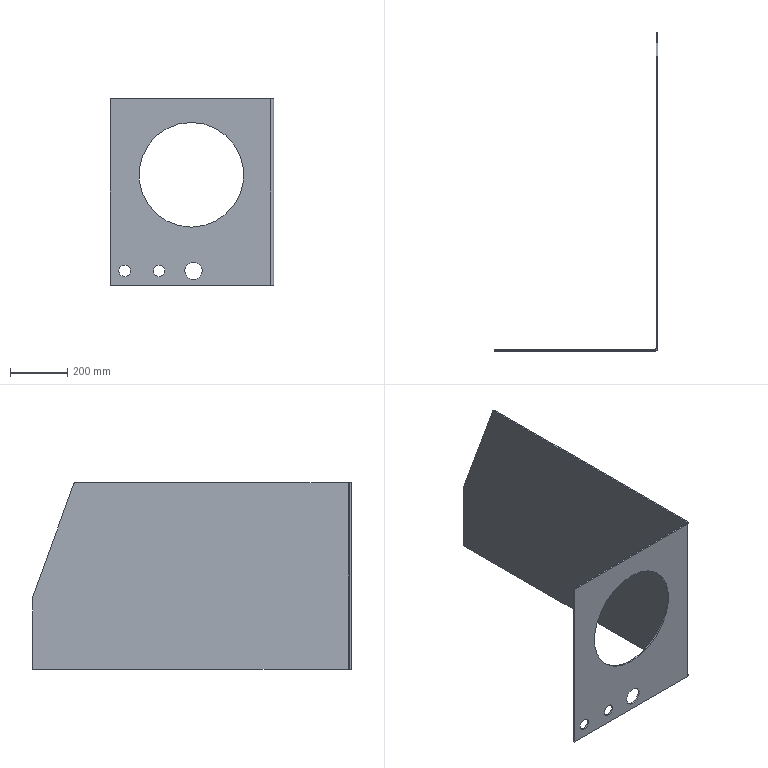Part | SolidWorks | features ICE 2, Fillet 1, FlatPattern 1, SMBaseFlange 1, SheetMetal 1, UnFold 1 | 1 solid | 25 faces | box 570.5 x 1110 x 651 mm | volume 4749925 mm3 | plane 13 | cylinder 12 | commonest cylinder face diameters 40 x4 12 x3 60 x2 365 x2 22 x1
STEP:
#1=CARTESIAN_POINT('',(50.5,5.,-295.));
#2=VERTEX_POINT('',#1);
#3=CARTESIAN_POINT('',(50.5,5.,-255.));
#4=VERTEX_POINT('',#3);
#5=CARTESIAN_POINT('',(50.5,5.,-275.));
#6=DIRECTION('',(0.,1.,0.));
#7=DIRECTION('',(0.,0.,1.));
#8=AXIS2_PLACEMENT_3D('',#5,#6,#7);
#9=CIRCLE('',#8,20.);
#10=EDGE_CURVE('',#2,#4,#9,.T.);
#11=ORIENTED_EDGE('',*,*,#10,.T.);
#12=CARTESIAN_POINT('',(50.5,0.,-255.));
#13=VERTEX_POINT('',#12);
#14=CARTESIAN_POINT('',(50.5,1110.5,-255.));
#15=DIRECTION('',(0.,-1.,0.));
#16=VECTOR('',#15,1000.);
#17=LINE('',#14,#16);
#18=EDGE_CURVE('',#4,#13,#17,.T.);
#19=ORIENTED_EDGE('',*,*,#18,.T.);
#20=CARTESIAN_POINT('',(50.5,0.,-295.));
#21=VERTEX_POINT('',#20);
#22=CARTESIAN_POINT('',(50.5,0.,-275.));
#23=DIRECTION('',(0.,-1.,0.));
#24=DIRECTION('',(0.,0.,-1.));
#25=AXIS2_PLACEMENT_3D('',#22,#23,#24);
#26=CIRCLE('',#25,20.);
#27=EDGE_CURVE('',#13,#21,#26,.T.);
#28=ORIENTED_EDGE('',*,*,#27,.T.);
#29=CARTESIAN_POINT('',(50.5,1110.5,-295.));
#30=DIRECTION('',(0.,-1.,0.));
#31=VECTOR('',#30,1000.);
#32=LINE('',#29,#31);
#33=EDGE_CURVE('',#2,#21,#32,.T.);
#34=ORIENTED_EDGE('',*,*,#33,.F.);
#35=EDGE_LOOP('',(#11,#19,#28,#34));
#36=FACE_OUTER_BOUND('',#35,.T.);
#37=CARTESIAN_POINT('',(50.5,1110.5,-275.));
#38=DIRECTION('',(0.,-1.,0.));
#39=DIRECTION('',(0.,0.,-1.));
#40=AXIS2_PLACEMENT_3D('',#37,#38,#39);
#41=CYLINDRICAL_SURFACE('',#40,20.);
#42=ADVANCED_FACE('',(#36),#41,.F.);
#43=CARTESIAN_POINT('',(170.5,5.,-295.));
#44=VERTEX_POINT('',#43);
#45=CARTESIAN_POINT('',(170.5,5.,-255.));
#46=VERTEX_POINT('',#45);
#47=CARTESIAN_POINT('',(170.5,5.,-275.));
#48=DIRECTION('',(0.,1.,0.));
#49=DIRECTION('',(0.,0.,1.));
#50=AXIS2_PLACEMENT_3D('',#47,#48,#49);
#51=CIRCLE('',#50,20.);
#52=EDGE_CURVE('',#44,#46,#51,.T.);
#53=ORIENTED_EDGE('',*,*,#52,.T.);
#54=CARTESIAN_POINT('',(170.5,0.,-255.));
#55=VERTEX_POINT('',#54);
#56=CARTESIAN_POINT('',(170.5,1110.5,-255.));
#57=DIRECTION('',(0.,-1.,0.));
#58=VECTOR('',#57,1000.);
#59=LINE('',#56,#58);
#60=EDGE_CURVE('',#46,#55,#59,.T.);
#61=ORIENTED_EDGE('',*,*,#60,.T.);
#62=CARTESIAN_POINT('',(170.5,0.,-295.));
#63=VERTEX_POINT('',#62);
#64=CARTESIAN_POINT('',(170.5,0.,-275.));
#65=DIRECTION('',(0.,-1.,0.));
#66=DIRECTION('',(0.,0.,-1.));
#67=AXIS2_PLACEMENT_3D('',#64,#65,#66);
#68=CIRCLE('',#67,20.);
#69=EDGE_CURVE('',#55,#63,#68,.T.);
#70=ORIENTED_EDGE('',*,*,#69,.T.);
#71=CARTESIAN_POINT('',(170.5,1110.5,-295.));
#72=DIRECTION('',(0.,-1.,0.));
#73=VECTOR('',#72,1000.);
#74=LINE('',#71,#73);
#75=EDGE_CURVE('',#44,#63,#74,.T.);
#76=ORIENTED_EDGE('',*,*,#75,.F.);
#77=EDGE_LOOP('',(#53,#61,#70,#76));
#78=FACE_OUTER_BOUND('',#77,.T.);
#79=CARTESIAN_POINT('',(170.5,1110.5,-275.));
#80=DIRECTION('',(0.,-1.,0.));
#81=DIRECTION('',(0.,0.,-1.));
#82=AXIS2_PLACEMENT_3D('',#79,#80,#81);
#83=CYLINDRICAL_SURFACE('',#82,20.);
#84=ADVANCED_FACE('',(#78),#83,.F.);
#85=CARTESIAN_POINT('',(290.5,5.,-305.));
#86=VERTEX_POINT('',#85);
#87=CARTESIAN_POINT('',(290.5,5.,-245.));
#88=VERTEX_POINT('',#87);
#89=CARTESIAN_POINT('',(290.5,5.,-275.));
#90=DIRECTION('',(0.,1.,0.));
#91=DIRECTION('',(0.,0.,1.));
#92=AXIS2_PLACEMENT_3D('',#89,#90,#91);
#93=CIRCLE('',#92,30.);
#94=EDGE_CURVE('',#86,#88,#93,.T.);
#95=ORIENTED_EDGE('',*,*,#94,.T.);
#96=CARTESIAN_POINT('',(290.5,0.,-245.));
#97=VERTEX_POINT('',#96);
#98=CARTESIAN_POINT('',(290.5,1110.5,-245.));
#99=DIRECTION('',(0.,-1.,0.));
#100=VECTOR('',#99,1000.);
#101=LINE('',#98,#100);
#102=EDGE_CURVE('',#88,#97,#101,.T.);
#103=ORIENTED_EDGE('',*,*,#102,.T.);
#104=CARTESIAN_POINT('',(290.5,0.,-305.));
#105=VERTEX_POINT('',#104);
#106=CARTESIAN_POINT('',(290.5,0.,-275.));
#107=DIRECTION('',(0.,-1.,0.));
#108=DIRECTION('',(0.,0.,-1.));
#109=AXIS2_PLACEMENT_3D('',#106,#107,#108);
#110=CIRCLE('',#109,30.);
#111=EDGE_CURVE('',#97,#105,#110,.T.);
#112=ORIENTED_EDGE('',*,*,#111,.T.);
#113=CARTESIAN_POINT('',(290.5,1110.5,-305.));
#114=DIRECTION('',(0.,-1.,0.));
#115=VECTOR('',#114,1000.);
#116=LINE('',#113,#115);
#117=EDGE_CURVE('',#86,#105,#116,.T.);
#118=ORIENTED_EDGE('',*,*,#117,.F.);
#119=EDGE_LOOP('',(#95,#103,#112,#118));
#120=FACE_OUTER_BOUND('',#119,.T.);
#121=CARTESIAN_POINT('',(290.5,1110.5,-275.));
#122=DIRECTION('',(0.,-1.,0.));
#123=DIRECTION('',(0.,0.,-1.));
#124=AXIS2_PLACEMENT_3D('',#121,#122,#123);
#125=CYLINDRICAL_SURFACE('',#124,30.);
#126=ADVANCED_FACE('',(#120),#125,.F.);
#127=CARTESIAN_POINT('',(283.,5.,-122.5));
#128=VERTEX_POINT('',#127);
#129=CARTESIAN_POINT('',(283.,5.,242.5));
#130=VERTEX_POINT('',#129);
#131=CARTESIAN_POINT('',(283.,5.,60.));
#132=DIRECTION('',(0.,1.,0.));
#133=DIRECTION('',(0.,0.,1.));
#134=AXIS2_PLACEMENT_3D('',#131,#132,#133);
#135=CIRCLE('',#134,182.5);
#136=EDGE_CURVE('',#128,#130,#135,.T.);
#137=ORIENTED_EDGE('',*,*,#136,.T.);
#138=CARTESIAN_POINT('',(283.,0.,242.5));
#139=VERTEX_POINT('',#138);
#140=CARTESIAN_POINT('',(283.,1110.5,242.5));
#141=DIRECTION('',(0.,-1.,0.));
#142=VECTOR('',#141,1000.);
#143=LINE('',#140,#142);
#144=EDGE_CURVE('',#130,#139,#143,.T.);
#145=ORIENTED_EDGE('',*,*,#144,.T.);
#146=CARTESIAN_POINT('',(283.,0.,-122.5));
#147=VERTEX_POINT('',#146);
#148=CARTESIAN_POINT('',(283.,0.,60.));
#149=DIRECTION('',(0.,-1.,0.));
#150=DIRECTION('',(0.,0.,-1.));
#151=AXIS2_PLACEMENT_3D('',#148,#149,#150);
#152=CIRCLE('',#151,182.5);
#153=EDGE_CURVE('',#139,#147,#152,.T.);
#154=ORIENTED_EDGE('',*,*,#153,.T.);
#155=CARTESIAN_POINT('',(283.,1110.5,-122.5));
#156=DIRECTION('',(0.,-1.,0.));
#157=VECTOR('',#156,1000.);
#158=LINE('',#155,#157);
#159=EDGE_CURVE('',#128,#147,#158,.T.);
#160=ORIENTED_EDGE('',*,*,#159,.F.);
#161=EDGE_LOOP('',(#137,#145,#154,#160));
#162=FACE_OUTER_BOUND('',#161,.T.);
#163=CARTESIAN_POINT('',(283.,1110.5,60.));
#164=DIRECTION('',(0.,-1.,0.));
#165=DIRECTION('',(0.,0.,-1.));
#166=AXIS2_PLACEMENT_3D('',#163,#164,#165);
#167=CYLINDRICAL_SURFACE('',#166,182.5);
#168=ADVANCED_FACE('',(#162),#167,.F.);
#169=CARTESIAN_POINT('',(559.5,0.,325.5));
#170=VERTEX_POINT('',#169);
#171=CARTESIAN_POINT('',(559.5,5.,325.5));
#172=VERTEX_POINT('',#171);
#173=CARTESIAN_POINT('',(559.5,0.,325.5));
#174=DIRECTION('',(0.,1.,0.));
#175=VECTOR('',#174,1000.);
#176=LINE('',#173,#175);
#177=EDGE_CURVE('',#170,#172,#176,.T.);
#178=ORIENTED_EDGE('',*,*,#177,.F.);
#179=CARTESIAN_POINT('',(570.5,11.,325.5));
#180=VERTEX_POINT('',#179);
#181=CARTESIAN_POINT('',(559.5,11.,325.5));
#182=DIRECTION('',(0.,0.,1.));
#183=DIRECTION('',(-1.,0.,0.));
#184=AXIS2_PLACEMENT_3D('',#181,#182,#183);
#185=CIRCLE('',#184,11.);
#186=EDGE_CURVE('',#170,#180,#185,.T.);
#187=ORIENTED_EDGE('',*,*,#186,.T.);
#188=CARTESIAN_POINT('',(565.5,11.,325.5));
#189=VERTEX_POINT('',#188);
#190=CARTESIAN_POINT('',(565.5,11.,325.5));
#191=DIRECTION('',(1.,0.,0.));
#192=VECTOR('',#191,1000.);
#193=LINE('',#190,#192);
#194=EDGE_CURVE('',#189,#180,#193,.T.);
#195=ORIENTED_EDGE('',*,*,#194,.F.);
#196=CARTESIAN_POINT('',(559.5,11.,325.5));
#197=DIRECTION('',(0.,0.,1.));
#198=DIRECTION('',(1.,0.,0.));
#199=AXIS2_PLACEMENT_3D('',#196,#197,#198);
#200=CIRCLE('',#199,6.);
#201=EDGE_CURVE('',#172,#189,#200,.T.);
#202=ORIENTED_EDGE('',*,*,#201,.F.);
#203=EDGE_LOOP('',(#178,#187,#195,#202));
#204=FACE_OUTER_BOUND('',#203,.T.);
#205=CARTESIAN_POINT('',(559.5,0.,325.5));
#206=DIRECTION('',(0.,0.,1.));
#207=DIRECTION('',(1.,0.,0.));
#208=AXIS2_PLACEMENT_3D('',#205,#206,#207);
#209=PLANE('',#208);
#210=ADVANCED_FACE('',(#204),#209,.T.);
#211=CARTESIAN_POINT('',(0.,0.,325.5));
#212=VERTEX_POINT('',#211);
#213=CARTESIAN_POINT('',(0.,0.,325.5));
#214=DIRECTION('',(1.,0.,0.));
#215=VECTOR('',#214,1000.);
#216=LINE('',#213,#215);
#217=EDGE_CURVE('',#212,#170,#216,.T.);
#218=ORIENTED_EDGE('',*,*,#217,.T.);
#219=ORIENTED_EDGE('',*,*,#177,.T.);
#220=CARTESIAN_POINT('',(0.,5.,325.5));
#221=VERTEX_POINT('',#220);
#222=CARTESIAN_POINT('',(0.,5.,325.5));
#223=DIRECTION('',(1.,0.,0.));
#224=VECTOR('',#223,1000.);
#225=LINE('',#222,#224);
#226=EDGE_CURVE('',#221,#172,#225,.T.);
#227=ORIENTED_EDGE('',*,*,#226,.F.);
#228=CARTESIAN_POINT('',(0.,0.,325.5));
#229=DIRECTION('',(0.,1.,0.));
#230=VECTOR('',#229,1000.);
#231=LINE('',#228,#230);
#232=EDGE_CURVE('',#212,#221,#231,.T.);
#233=ORIENTED_EDGE('',*,*,#232,.F.);
#234=EDGE_LOOP('',(#218,#219,#227,#233));
#235=FACE_OUTER_BOUND('',#234,.T.);
#236=CARTESIAN_POINT('',(565.5,11.,325.5));
#237=DIRECTION('',(0.,0.,1.));
#238=DIRECTION('',(1.,0.,0.));
#239=AXIS2_PLACEMENT_3D('',#236,#237,#238);
#240=PLANE('',#239);
#241=ADVANCED_FACE('',(#235),#240,.T.);
#242=CARTESIAN_POINT('',(570.5,11.,-325.5));
#243=VERTEX_POINT('',#242);
#244=CARTESIAN_POINT('',(565.5,11.,-325.5));
#245=VERTEX_POINT('',#244);
#246=CARTESIAN_POINT('',(570.5,11.,-325.5));
#247=DIRECTION('',(-1.,0.,0.));
#248=VECTOR('',#247,1000.);
#249=LINE('',#246,#248);
#250=EDGE_CURVE('',#243,#245,#249,.T.);
#251=ORIENTED_EDGE('',*,*,#250,.F.);
#252=CARTESIAN_POINT('',(559.5,0.,-325.5));
#253=VERTEX_POINT('',#252);
#254=CARTESIAN_POINT('',(559.5,11.,-325.5));
#255=DIRECTION('',(0.,0.,1.));
#256=DIRECTION('',(-1.,0.,0.));
#257=AXIS2_PLACEMENT_3D('',#254,#255,#256);
#258=CIRCLE('',#257,11.);
#259=EDGE_CURVE('',#253,#243,#258,.T.);
#260=ORIENTED_EDGE('',*,*,#259,.F.);
#261=CARTESIAN_POINT('',(559.5,5.,-325.5));
#262=VERTEX_POINT('',#261);
#263=CARTESIAN_POINT('',(559.5,5.,-325.5));
#264=DIRECTION('',(0.,-1.,0.));
#265=VECTOR('',#264,1000.);
#266=LINE('',#263,#265);
#267=EDGE_CURVE('',#262,#253,#266,.T.);
#268=ORIENTED_EDGE('',*,*,#267,.F.);
#269=CARTESIAN_POINT('',(559.5,11.,-325.5));
#270=DIRECTION('',(0.,0.,1.));
#271=DIRECTION('',(1.,0.,0.));
#272=AXIS2_PLACEMENT_3D('',#269,#270,#271);
#273=CIRCLE('',#272,6.);
#274=EDGE_CURVE('',#262,#245,#273,.T.);
#275=ORIENTED_EDGE('',*,*,#274,.T.);
#276=EDGE_LOOP('',(#251,#260,#268,#275));
#277=FACE_OUTER_BOUND('',#276,.T.);
#278=CARTESIAN_POINT('',(570.5,11.,-325.5));
#279=DIRECTION('',(0.,0.,-1.));
#280=DIRECTION('',(-1.,0.,0.));
#281=AXIS2_PLACEMENT_3D('',#278,#279,#280);
#282=PLANE('',#281);
#283=ADVANCED_FACE('',(#277),#282,.T.);
#284=CARTESIAN_POINT('',(570.5,1110.5,-325.5));
#285=VERTEX_POINT('',#284);
#286=CARTESIAN_POINT('',(570.5,0.,-325.5));
#287=DIRECTION('',(0.,1.,0.));
#288=VECTOR('',#287,1000.);
#289=LINE('',#286,#288);
#290=EDGE_CURVE('',#243,#285,#289,.T.);
#291=ORIENTED_EDGE('',*,*,#290,.F.);
#292=ORIENTED_EDGE('',*,*,#250,.T.);
#293=CARTESIAN_POINT('',(565.5,1110.5,-325.5));
#294=VERTEX_POINT('',#293);
#295=CARTESIAN_POINT('',(565.5,0.,-325.5));
#296=DIRECTION('',(0.,1.,0.));
#297=VECTOR('',#296,1000.);
#298=LINE('',#295,#297);
#299=EDGE_CURVE('',#245,#294,#298,.T.);
#300=ORIENTED_EDGE('',*,*,#299,.T.);
#301=CARTESIAN_POINT('',(565.5,1110.5,-325.5));
#302=DIRECTION('',(1.,0.,0.));
#303=VECTOR('',#302,1000.);
#304=LINE('',#301,#303);
#305=EDGE_CURVE('',#294,#285,#304,.T.);
#306=ORIENTED_EDGE('',*,*,#305,.T.);
#307=EDGE_LOOP('',(#291,#292,#300,#306));
#308=FACE_OUTER_BOUND('',#307,.T.);
#309=CARTESIAN_POINT('',(559.5,5.,-325.5));
#310=DIRECTION('',(0.,0.,-1.));
#311=DIRECTION('',(-1.,0.,0.));
#312=AXIS2_PLACEMENT_3D('',#309,#310,#311);
#313=PLANE('',#312);
#314=ADVANCED_FACE('',(#308),#313,.T.);
#315=CARTESIAN_POINT('',(570.5,1110.5,-72.938));
#316=VERTEX_POINT('',#315);
#317=CARTESIAN_POINT('',(570.5,1110.5,325.5));
#318=DIRECTION('',(0.,0.,-1.));
#319=VECTOR('',#318,1000.);
#320=LINE('',#317,#319);
#321=EDGE_CURVE('',#316,#285,#320,.T.);
#322=ORIENTED_EDGE('',*,*,#321,.F.);
#323=CARTESIAN_POINT('',(570.5,1110.138,-70.886));
#324=VERTEX_POINT('',#323);
#325=CARTESIAN_POINT('',(570.5,1104.5,-72.938));
#326=DIRECTION('',(1.,0.,0.));
#327=DIRECTION('',(0.,0.,1.));
#328=AXIS2_PLACEMENT_3D('',#325,#326,#327);
#329=CIRCLE('',#328,6.);
#330=EDGE_CURVE('',#316,#324,#329,.T.);
#331=ORIENTED_EDGE('',*,*,#330,.T.);
#332=CARTESIAN_POINT('',(570.5,967.302,321.552));
#333=VERTEX_POINT('',#332);
#334=CARTESIAN_POINT('',(570.5,1110.5,-71.88));
#335=DIRECTION('',(0.,0.342,-0.9397));
#336=VECTOR('',#335,1000.);
#337=LINE('',#334,#336);
#338=EDGE_CURVE('',#333,#324,#337,.T.);
#339=ORIENTED_EDGE('',*,*,#338,.F.);
#340=CARTESIAN_POINT('',(570.5,961.664,325.5));
#341=VERTEX_POINT('',#340);
#342=CARTESIAN_POINT('',(570.5,961.664,319.5));
#343=DIRECTION('',(1.,0.,0.));
#344=DIRECTION('',(0.,0.,1.));
#345=AXIS2_PLACEMENT_3D('',#342,#343,#344);
#346=CIRCLE('',#345,6.);
#347=EDGE_CURVE('',#333,#341,#346,.T.);
#348=ORIENTED_EDGE('',*,*,#347,.T.);
#349=CARTESIAN_POINT('',(570.5,0.,325.5));
#350=DIRECTION('',(0.,1.,0.));
#351=VECTOR('',#350,1000.);
#352=LINE('',#349,#351);
#353=EDGE_CURVE('',#180,#341,#352,.T.);
#354=ORIENTED_EDGE('',*,*,#353,.F.);
#355=CARTESIAN_POINT('',(570.5,11.,325.5));
#356=DIRECTION('',(0.,0.,-1.));
#357=VECTOR('',#356,1000.);
#358=LINE('',#355,#357);
#359=EDGE_CURVE('',#180,#243,#358,.T.);
#360=ORIENTED_EDGE('',*,*,#359,.T.);
#361=ORIENTED_EDGE('',*,*,#290,.T.);
#362=EDGE_LOOP('',(#322,#331,#339,#348,#354,#360,#361));
#363=FACE_OUTER_BOUND('',#362,.T.);
#364=CARTESIAN_POINT('',(570.5,0.,325.5));
#365=DIRECTION('',(-1.,0.,0.));
#366=DIRECTION('',(0.,0.,1.));
#367=AXIS2_PLACEMENT_3D('',#364,#365,#366);
#368=PLANE('',#367);
#369=ADVANCED_FACE('',(#363),#368,.F.);
#370=CARTESIAN_POINT('',(565.5,1110.5,-72.938));
#371=VERTEX_POINT('',#370);
#372=CARTESIAN_POINT('',(565.5,1110.5,325.5));
#373=DIRECTION('',(0.,0.,-1.));
#374=VECTOR('',#373,1000.);
#375=LINE('',#372,#374);
#376=EDGE_CURVE('',#371,#294,#375,.T.);
#377=ORIENTED_EDGE('',*,*,#376,.F.);
#378=CARTESIAN_POINT('',(570.5,1110.5,-72.938));
#379=DIRECTION('',(1.,0.,0.));
#380=VECTOR('',#379,1000.);
#381=LINE('',#378,#380);
#382=EDGE_CURVE('',#371,#316,#381,.T.);
#383=ORIENTED_EDGE('',*,*,#382,.T.);
#384=ORIENTED_EDGE('',*,*,#321,.T.);
#385=ORIENTED_EDGE('',*,*,#305,.F.);
#386=EDGE_LOOP('',(#377,#383,#384,#385));
#387=FACE_OUTER_BOUND('',#386,.T.);
#388=CARTESIAN_POINT('',(565.5,1110.5,325.5));
#389=DIRECTION('',(0.,1.,0.));
#390=DIRECTION('',(0.,0.,1.));
#391=AXIS2_PLACEMENT_3D('',#388,#389,#390);
#392=PLANE('',#391);
#393=ADVANCED_FACE('',(#387),#392,.T.);
#394=CARTESIAN_POINT('',(565.5,1110.138,-70.886));
#395=VERTEX_POINT('',#394);
#396=CARTESIAN_POINT('',(565.5,967.302,321.552));
#397=VERTEX_POINT('',#396);
#398=CARTESIAN_POINT('',(565.5,852.881,635.923));
#399=DIRECTION('',(0.,-0.342,0.9397));
#400=VECTOR('',#399,1000.);
#401=LINE('',#398,#400);
#402=EDGE_CURVE('',#395,#397,#401,.T.);
#403=ORIENTED_EDGE('',*,*,#402,.F.);
#404=CARTESIAN_POINT('',(565.5,1104.5,-72.938));
#405=DIRECTION('',(-1.,0.,0.));
#406=DIRECTION('',(0.,0.,1.));
#407=AXIS2_PLACEMENT_3D('',#404,#405,#406);
#408=CIRCLE('',#407,6.);
#409=EDGE_CURVE('',#395,#371,#408,.T.);
#410=ORIENTED_EDGE('',*,*,#409,.T.);
#411=ORIENTED_EDGE('',*,*,#376,.T.);
#412=ORIENTED_EDGE('',*,*,#299,.F.);
#413=CARTESIAN_POINT('',(565.5,11.,325.5));
#414=DIRECTION('',(0.,0.,-1.));
#415=VECTOR('',#414,1000.);
#416=LINE('',#413,#415);
#417=EDGE_CURVE('',#189,#245,#416,.T.);
#418=ORIENTED_EDGE('',*,*,#417,.F.);
#419=CARTESIAN_POINT('',(565.5,961.664,325.5));
#420=VERTEX_POINT('',#419);
#421=CARTESIAN_POINT('',(565.5,0.,325.5));
#422=DIRECTION('',(0.,1.,0.));
#423=VECTOR('',#422,1000.);
#424=LINE('',#421,#423);
#425=EDGE_CURVE('',#189,#420,#424,.T.);
#426=ORIENTED_EDGE('',*,*,#425,.T.);
#427=CARTESIAN_POINT('',(565.5,961.664,319.5));
#428=DIRECTION('',(-1.,0.,0.));
#429=DIRECTION('',(0.,0.,1.));
#430=AXIS2_PLACEMENT_3D('',#427,#428,#429);
#431=CIRCLE('',#430,6.);
#432=EDGE_CURVE('',#420,#397,#431,.T.);
#433=ORIENTED_EDGE('',*,*,#432,.T.);
#434=EDGE_LOOP('',(#403,#410,#411,#412,#418,#426,#433));
#435=FACE_OUTER_BOUND('',#434,.T.);
#436=CARTESIAN_POINT('',(565.5,0.,325.5));
#437=DIRECTION('',(-1.,0.,0.));
#438=DIRECTION('',(0.,0.,1.));
#439=AXIS2_PLACEMENT_3D('',#436,#437,#438);
#440=PLANE('',#439);
#441=ADVANCED_FACE('',(#435),#440,.T.);
#442=ORIENTED_EDGE('',*,*,#274,.F.);
#443=CARTESIAN_POINT('',(559.5,5.,325.5));
#444=DIRECTION('',(0.,0.,-1.));
#445=VECTOR('',#444,1000.);
#446=LINE('',#443,#445);
#447=EDGE_CURVE('',#172,#262,#446,.T.);
#448=ORIENTED_EDGE('',*,*,#447,.F.);
#449=ORIENTED_EDGE('',*,*,#201,.T.);
#450=ORIENTED_EDGE('',*,*,#417,.T.);
#451=EDGE_LOOP('',(#442,#448,#449,#450));
#452=FACE_OUTER_BOUND('',#451,.T.);
#453=CARTESIAN_POINT('',(559.5,11.,325.5));
#454=DIRECTION('',(0.,0.,-1.));
#455=DIRECTION('',(-1.,0.,0.));
#456=AXIS2_PLACEMENT_3D('',#453,#454,#455);
#457=CYLINDRICAL_SURFACE('',#456,6.);
#458=ADVANCED_FACE('',(#452),#457,.F.);
#459=ORIENTED_EDGE('',*,*,#10,.F.);
#460=CARTESIAN_POINT('',(50.5,5.,-275.));
#461=DIRECTION('',(0.,1.,0.));
#462=DIRECTION('',(0.,0.,1.));
#463=AXIS2_PLACEMENT_3D('',#460,#461,#462);
#464=CIRCLE('',#463,20.);
#465=EDGE_CURVE('',#4,#2,#464,.T.);
#466=ORIENTED_EDGE('',*,*,#465,.F.);
#467=EDGE_LOOP('',(#459,#466));
#468=FACE_BOUND('',#467,.T.);
#469=ORIENTED_EDGE('',*,*,#52,.F.);
#470=CARTESIAN_POINT('',(170.5,5.,-275.));
#471=DIRECTION('',(0.,1.,0.));
#472=DIRECTION('',(0.,0.,1.));
#473=AXIS2_PLACEMENT_3D('',#470,#471,#472);
#474=CIRCLE('',#473,20.);
#475=EDGE_CURVE('',#46,#44,#474,.T.);
#476=ORIENTED_EDGE('',*,*,#475,.F.);
#477=EDGE_LOOP('',(#469,#476));
#478=FACE_BOUND('',#477,.T.);
#479=ORIENTED_EDGE('',*,*,#94,.F.);
#480=CARTESIAN_POINT('',(290.5,5.,-275.));
#481=DIRECTION('',(0.,1.,0.));
#482=DIRECTION('',(0.,0.,1.));
#483=AXIS2_PLACEMENT_3D('',#480,#481,#482);
#484=CIRCLE('',#483,30.);
#485=EDGE_CURVE('',#88,#86,#484,.T.);
#486=ORIENTED_EDGE('',*,*,#485,.F.);
#487=EDGE_LOOP('',(#479,#486));
#488=FACE_BOUND('',#487,.T.);
#489=ORIENTED_EDGE('',*,*,#136,.F.);
#490=CARTESIAN_POINT('',(283.,5.,60.));
#491=DIRECTION('',(0.,1.,0.));
#492=DIRECTION('',(0.,0.,1.));
#493=AXIS2_PLACEMENT_3D('',#490,#491,#492);
#494=CIRCLE('',#493,182.5);
#495=EDGE_CURVE('',#130,#128,#494,.T.);
#496=ORIENTED_EDGE('',*,*,#495,.F.);
#497=EDGE_LOOP('',(#489,#496));
#498=FACE_BOUND('',#497,.T.);
#499=CARTESIAN_POINT('',(0.,5.,-325.5));
#500=VERTEX_POINT('',#499);
#501=CARTESIAN_POINT('',(0.,5.,-325.5));
#502=DIRECTION('',(1.,0.,0.));
#503=VECTOR('',#502,1000.);
#504=LINE('',#501,#503);
#505=EDGE_CURVE('',#500,#262,#504,.T.);
#506=ORIENTED_EDGE('',*,*,#505,.F.);
#507=CARTESIAN_POINT('',(0.,5.,325.5));
#508=DIRECTION('',(0.,0.,-1.));
#509=VECTOR('',#508,1000.);
#510=LINE('',#507,#509);
#511=EDGE_CURVE('',#221,#500,#510,.T.);
#512=ORIENTED_EDGE('',*,*,#511,.F.);
#513=ORIENTED_EDGE('',*,*,#226,.T.);
#514=ORIENTED_EDGE('',*,*,#447,.T.);
#515=EDGE_LOOP('',(#506,#512,#513,#514));
#516=FACE_OUTER_BOUND('',#515,.T.);
#517=CARTESIAN_POINT('',(0.,5.,325.5));
#518=DIRECTION('',(0.,1.,0.));
#519=DIRECTION('',(0.,0.,1.));
#520=AXIS2_PLACEMENT_3D('',#517,#518,#519);
#521=PLANE('',#520);
#522=ADVANCED_FACE('',(#468,#478,#488,#498,#516),#521,.T.);
#523=CARTESIAN_POINT('',(0.,0.,-325.5));
#524=VERTEX_POINT('',#523);
#525=CARTESIAN_POINT('',(0.,0.,-325.5));
#526=DIRECTION('',(0.,1.,0.));
#527=VECTOR('',#526,1000.);
#528=LINE('',#525,#527);
#529=EDGE_CURVE('',#524,#500,#528,.T.);
#530=ORIENTED_EDGE('',*,*,#529,.F.);
#531=CARTESIAN_POINT('',(0.,0.,325.5));
#532=DIRECTION('',(0.,0.,-1.));
#533=VECTOR('',#532,1000.);
#534=LINE('',#531,#533);
#535=EDGE_CURVE('',#212,#524,#534,.T.);
#536=ORIENTED_EDGE('',*,*,#535,.F.);
#537=ORIENTED_EDGE('',*,*,#232,.T.);
#538=ORIENTED_EDGE('',*,*,#511,.T.);
#539=EDGE_LOOP('',(#530,#536,#537,#538));
#540=FACE_OUTER_BOUND('',#539,.T.);
#541=CARTESIAN_POINT('',(0.,0.,325.5));
#542=DIRECTION('',(-1.,0.,0.));
#543=DIRECTION('',(0.,0.,1.));
#544=AXIS2_PLACEMENT_3D('',#541,#542,#543);
#545=PLANE('',#544);
#546=ADVANCED_FACE('',(#540),#545,.T.);
#547=CARTESIAN_POINT('',(50.5,0.,-275.));
#548=DIRECTION('',(0.,-1.,0.));
#549=DIRECTION('',(0.,0.,-1.));
#550=AXIS2_PLACEMENT_3D('',#547,#548,#549);
#551=CIRCLE('',#550,20.);
#552=EDGE_CURVE('',#21,#13,#551,.T.);
#553=ORIENTED_EDGE('',*,*,#552,.F.);
#554=ORIENTED_EDGE('',*,*,#27,.F.);
#555=EDGE_LOOP('',(#553,#554));
#556=FACE_BOUND('',#555,.T.);
#557=CARTESIAN_POINT('',(170.5,0.,-275.));
#558=DIRECTION('',(0.,-1.,0.));
#559=DIRECTION('',(0.,0.,-1.));
#560=AXIS2_PLACEMENT_3D('',#557,#558,#559);
#561=CIRCLE('',#560,20.);
#562=EDGE_CURVE('',#63,#55,#561,.T.);
#563=ORIENTED_EDGE('',*,*,#562,.F.);
#564=ORIENTED_EDGE('',*,*,#69,.F.);
#565=EDGE_LOOP('',(#563,#564));
#566=FACE_BOUND('',#565,.T.);
#567=CARTESIAN_POINT('',(290.5,0.,-275.));
#568=DIRECTION('',(0.,-1.,0.));
#569=DIRECTION('',(0.,0.,-1.));
#570=AXIS2_PLACEMENT_3D('',#567,#568,#569);
#571=CIRCLE('',#570,30.);
#572=EDGE_CURVE('',#105,#97,#571,.T.);
#573=ORIENTED_EDGE('',*,*,#572,.F.);
#574=ORIENTED_EDGE('',*,*,#111,.F.);
#575=EDGE_LOOP('',(#573,#574));
#576=FACE_BOUND('',#575,.T.);
#577=CARTESIAN_POINT('',(283.,0.,60.));
#578=DIRECTION('',(0.,-1.,0.));
#579=DIRECTION('',(0.,0.,-1.));
#580=AXIS2_PLACEMENT_3D('',#577,#578,#579);
#581=CIRCLE('',#580,182.5);
#582=EDGE_CURVE('',#147,#139,#581,.T.);
#583=ORIENTED_EDGE('',*,*,#582,.F.);
#584=ORIENTED_EDGE('',*,*,#153,.F.);
#585=EDGE_LOOP('',(#583,#584));
#586=FACE_BOUND('',#585,.T.);
#587=CARTESIAN_POINT('',(0.,0.,-325.5));
#588=DIRECTION('',(1.,0.,0.));
#589=VECTOR('',#588,1000.);
#590=LINE('',#587,#589);
#591=EDGE_CURVE('',#524,#253,#590,.T.);
#592=ORIENTED_EDGE('',*,*,#591,.T.);
#593=CARTESIAN_POINT('',(559.5,0.,325.5));
#594=DIRECTION('',(0.,0.,-1.));
#595=VECTOR('',#594,1000.);
#596=LINE('',#593,#595);
#597=EDGE_CURVE('',#170,#253,#596,.T.);
#598=ORIENTED_EDGE('',*,*,#597,.F.);
#599=ORIENTED_EDGE('',*,*,#217,.F.);
#600=ORIENTED_EDGE('',*,*,#535,.T.);
#601=EDGE_LOOP('',(#592,#598,#599,#600));
#602=FACE_OUTER_BOUND('',#601,.T.);
#603=CARTESIAN_POINT('',(0.,0.,325.5));
#604=DIRECTION('',(0.,1.,0.));
#605=DIRECTION('',(0.,0.,1.));
#606=AXIS2_PLACEMENT_3D('',#603,#604,#605);
#607=PLANE('',#606);
#608=ADVANCED_FACE('',(#556,#566,#576,#586,#602),#607,.F.);
#609=ORIENTED_EDGE('',*,*,#259,.T.);
#610=ORIENTED_EDGE('',*,*,#359,.F.);
#611=ORIENTED_EDGE('',*,*,#186,.F.);
#612=ORIENTED_EDGE('',*,*,#597,.T.);
#613=EDGE_LOOP('',(#609,#610,#611,#612));
#614=FACE_OUTER_BOUND('',#613,.T.);
#615=CARTESIAN_POINT('',(559.5,11.,325.5));
#616=DIRECTION('',(0.,0.,-1.));
#617=DIRECTION('',(-1.,0.,0.));
#618=AXIS2_PLACEMENT_3D('',#615,#616,#617);
#619=CYLINDRICAL_SURFACE('',#618,11.);
#620=ADVANCED_FACE('',(#614),#619,.T.);
#621=ORIENTED_EDGE('',*,*,#353,.T.);
#622=CARTESIAN_POINT('',(565.5,961.664,325.5));
#623=DIRECTION('',(-1.,0.,0.));
#624=VECTOR('',#623,1000.);
#625=LINE('',#622,#624);
#626=EDGE_CURVE('',#341,#420,#625,.T.);
#627=ORIENTED_EDGE('',*,*,#626,.T.);
#628=ORIENTED_EDGE('',*,*,#425,.F.);
#629=ORIENTED_EDGE('',*,*,#194,.T.);
#630=EDGE_LOOP('',(#621,#627,#628,#629));
#631=FACE_OUTER_BOUND('',#630,.T.);
#632=CARTESIAN_POINT('',(559.5,11.,325.5));
#633=DIRECTION('',(0.,0.,1.));
#634=DIRECTION('',(1.,0.,0.));
#635=AXIS2_PLACEMENT_3D('',#632,#633,#634);
#636=PLANE('',#635);
#637=ADVANCED_FACE('',(#631),#636,.T.);
#638=ORIENTED_EDGE('',*,*,#505,.T.);
#639=ORIENTED_EDGE('',*,*,#267,.T.);
#640=ORIENTED_EDGE('',*,*,#591,.F.);
#641=ORIENTED_EDGE('',*,*,#529,.T.);
#642=EDGE_LOOP('',(#638,#639,#640,#641));
#643=FACE_OUTER_BOUND('',#642,.T.);
#644=CARTESIAN_POINT('',(559.5,11.,-325.5));
#645=DIRECTION('',(0.,0.,1.));
#646=DIRECTION('',(1.,0.,0.));
#647=AXIS2_PLACEMENT_3D('',#644,#645,#646);
#648=PLANE('',#647);
#649=ADVANCED_FACE('',(#643),#648,.F.);
#650=ORIENTED_EDGE('',*,*,#338,.T.);
#651=CARTESIAN_POINT('',(565.5,1110.138,-70.886));
#652=DIRECTION('',(-1.,0.,0.));
#653=VECTOR('',#652,1000.);
#654=LINE('',#651,#653);
#655=EDGE_CURVE('',#324,#395,#654,.T.);
#656=ORIENTED_EDGE('',*,*,#655,.T.);
#657=ORIENTED_EDGE('',*,*,#402,.T.);
#658=CARTESIAN_POINT('',(570.5,967.302,321.552));
#659=DIRECTION('',(1.,0.,0.));
#660=VECTOR('',#659,1000.);
#661=LINE('',#658,#660);
#662=EDGE_CURVE('',#397,#333,#661,.T.);
#663=ORIENTED_EDGE('',*,*,#662,.T.);
#664=EDGE_LOOP('',(#650,#656,#657,#663));
#665=FACE_OUTER_BOUND('',#664,.T.);
#666=CARTESIAN_POINT('',(0.,1110.5,-71.88));
#667=DIRECTION('',(0.,-0.9397,-0.342));
#668=DIRECTION('',(0.,0.342,-0.9397));
#669=AXIS2_PLACEMENT_3D('',#666,#667,#668);
#670=PLANE('',#669);
#671=ADVANCED_FACE('',(#665),#670,.F.);
#672=ORIENTED_EDGE('',*,*,#409,.F.);
#673=ORIENTED_EDGE('',*,*,#655,.F.);
#674=ORIENTED_EDGE('',*,*,#330,.F.);
#675=ORIENTED_EDGE('',*,*,#382,.F.);
#676=EDGE_LOOP('',(#672,#673,#674,#675));
#677=FACE_OUTER_BOUND('',#676,.T.);
#678=CARTESIAN_POINT('',(565.5,1104.5,-72.938));
#679=DIRECTION('',(-1.,0.,0.));
#680=DIRECTION('',(0.,0.,1.));
#681=AXIS2_PLACEMENT_3D('',#678,#679,#680);
#682=CYLINDRICAL_SURFACE('',#681,6.);
#683=ADVANCED_FACE('',(#677),#682,.T.);
#684=ORIENTED_EDGE('',*,*,#432,.F.);
#685=ORIENTED_EDGE('',*,*,#626,.F.);
#686=ORIENTED_EDGE('',*,*,#347,.F.);
#687=ORIENTED_EDGE('',*,*,#662,.F.);
#688=EDGE_LOOP('',(#684,#685,#686,#687));
#689=FACE_OUTER_BOUND('',#688,.T.);
#690=CARTESIAN_POINT('',(0.,961.664,319.5));
#691=DIRECTION('',(-1.,0.,0.));
#692=DIRECTION('',(0.,0.,1.));
#693=AXIS2_PLACEMENT_3D('',#690,#691,#692);
#694=CYLINDRICAL_SURFACE('',#693,6.);
#695=ADVANCED_FACE('',(#689),#694,.T.);
#696=ORIENTED_EDGE('',*,*,#144,.F.);
#697=ORIENTED_EDGE('',*,*,#495,.T.);
#698=ORIENTED_EDGE('',*,*,#159,.T.);
#699=ORIENTED_EDGE('',*,*,#582,.T.);
#700=EDGE_LOOP('',(#696,#697,#698,#699));
#701=FACE_OUTER_BOUND('',#700,.T.);
#702=CARTESIAN_POINT('',(283.,1110.5,60.));
#703=DIRECTION('',(0.,-1.,0.));
#704=DIRECTION('',(0.,0.,-1.));
#705=AXIS2_PLACEMENT_3D('',#702,#703,#704);
#706=CYLINDRICAL_SURFACE('',#705,182.5);
#707=ADVANCED_FACE('',(#701),#706,.F.);
#708=ORIENTED_EDGE('',*,*,#102,.F.);
#709=ORIENTED_EDGE('',*,*,#485,.T.);
#710=ORIENTED_EDGE('',*,*,#117,.T.);
#711=ORIENTED_EDGE('',*,*,#572,.T.);
#712=EDGE_LOOP('',(#708,#709,#710,#711));
#713=FACE_OUTER_BOUND('',#712,.T.);
#714=CARTESIAN_POINT('',(290.5,1110.5,-275.));
#715=DIRECTION('',(0.,-1.,0.));
#716=DIRECTION('',(0.,0.,-1.));
#717=AXIS2_PLACEMENT_3D('',#714,#715,#716);
#718=CYLINDRICAL_SURFACE('',#717,30.);
#719=ADVANCED_FACE('',(#713),#718,.F.);
#720=ORIENTED_EDGE('',*,*,#60,.F.);
#721=ORIENTED_EDGE('',*,*,#475,.T.);
#722=ORIENTED_EDGE('',*,*,#75,.T.);
#723=ORIENTED_EDGE('',*,*,#562,.T.);
#724=EDGE_LOOP('',(#720,#721,#722,#723));
#725=FACE_OUTER_BOUND('',#724,.T.);
#726=CARTESIAN_POINT('',(170.5,1110.5,-275.));
#727=DIRECTION('',(0.,-1.,0.));
#728=DIRECTION('',(0.,0.,-1.));
#729=AXIS2_PLACEMENT_3D('',#726,#727,#728);
#730=CYLINDRICAL_SURFACE('',#729,20.);
#731=ADVANCED_FACE('',(#725),#730,.F.);
#732=ORIENTED_EDGE('',*,*,#18,.F.);
#733=ORIENTED_EDGE('',*,*,#465,.T.);
#734=ORIENTED_EDGE('',*,*,#33,.T.);
#735=ORIENTED_EDGE('',*,*,#552,.T.);
#736=EDGE_LOOP('',(#732,#733,#734,#735));
#737=FACE_OUTER_BOUND('',#736,.T.);
#738=CARTESIAN_POINT('',(50.5,1110.5,-275.));
#739=DIRECTION('',(0.,-1.,0.));
#740=DIRECTION('',(0.,0.,-1.));
#741=AXIS2_PLACEMENT_3D('',#738,#739,#740);
#742=CYLINDRICAL_SURFACE('',#741,20.);
#743=ADVANCED_FACE('',(#737),#742,.F.);
#744=CLOSED_SHELL('',(#42,#84,#126,#168,#210,#241,#283,#314,#369,#393,#441,#458,#522,#546,#608,#620,#637,#649,#671,#683,#695,#707,#719,#731,#743));
#745=MANIFOLD_SOLID_BREP('',#744);
#746=CARTESIAN_POINT('',(0.,0.,0.));
#747=DIRECTION('',(0.,0.,1.));
#748=DIRECTION('',(1.,0.,0.));
#749=AXIS2_PLACEMENT_3D('',#746,#747,#748);
#750=(LENGTH_UNIT()NAMED_UNIT(*)SI_UNIT(.MILLI.,.METRE.));
#751=UNCERTAINTY_MEASURE_WITH_UNIT(LENGTH_MEASURE(0.00001),#750,'','');
#752=(NAMED_UNIT(*)PLANE_ANGLE_UNIT()SI_UNIT($,.RADIAN.));
#753=(NAMED_UNIT(*)SI_UNIT($,.STERADIAN.)SOLID_ANGLE_UNIT());
#754=(GEOMETRIC_REPRESENTATION_CONTEXT(3)GLOBAL_UNCERTAINTY_ASSIGNED_CONTEXT((#751))GLOBAL_UNIT_ASSIGNED_CONTEXT((#750,#752,#753))REPRESENTATION_CONTEXT('',''));
#755=ADVANCED_BREP_SHAPE_REPRESENTATION('',(#745,#749),#754);